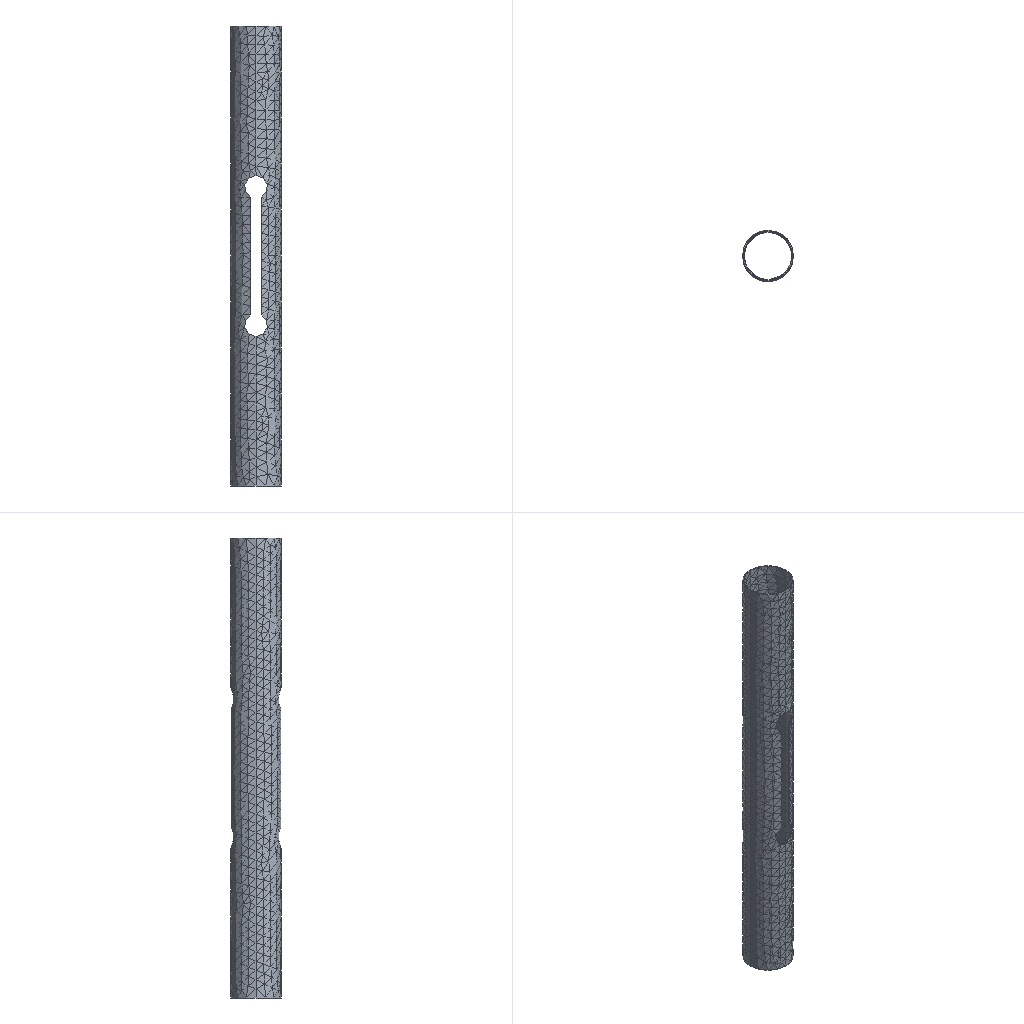Simulation study | abaqus
Set-up summary:
category,name,step,type,value,unit,region
solver,abaqus,,Abaqus/CAE 2024
units,mm-N-s-tonne (MPa),,inferred,E=210000 density=7.85e-09
analysis,Pinch_Step,,dynamic explicit,nlgeom=True; time_period=0.01
mesh,nodes,,,2587
mesh,elements,,,5865
element_type,C3D4,,,5022
element_type,R3D4,,,795
element_type,R3D3,,,48
material,Material-1,,E,210000
material,Material-1,,nu,0.3
material,Material-1,,density,7.85e-09
material,Material-1,,yield,1000
material,Material-1,,behaviors,plastic
section,Material-1,,solid section,,,Set-11
bc,BC-Deploy,Pinch_Step,fixed,"[dofs=x,y n=2]",,Set-9
bc,BC-Pinch_niehe,Pinch_Step,displacement,-60 [dofs=x],,Set-5
bc,BC-Pinch_niehe,Pinch_Step,fixed,"[dofs=rx,ry,rz,y,z n=5]",,Set-5
contact,Int-2,initial,general contact,interaction=IntProp-1; friction=0; behavior=hard
contact,Int-1,Pinch_Step,contact pair,interaction=IntProp-1; friction=0; behavior=hard,,jiaolian-waibiaomian / xinban-waibiaomian
constraint,rigid body,,,1
Abaqus input file, long lists of numbers shortened:
*Heading
** Job name: deck Model name: yuanjiaolian-Copy
** Generated by: Abaqus/CAE 2024
*Preprint, echo=NO, model=NO, history=NO, contact=NO
**
** PARTS
**
*Part, name=jiaolian11
*Node
      1, -2.39031069e-05,         -5.5,         100.
      2, -2.45171304e-05,        -5.25,         100.
** (1765 more lines like these left out)
*Element, type=C3D4
   1, 1763,  733,  592,   88
   2, 1763,   88,    6,   89
** (5020 more lines like these left out)
*Nset, nset=Set-11, generate
    1,  1767,     1
*Elset, elset=Set-11, generate
    1,  5022,     1
** Section: Section-2
*Solid Section, elset=Set-11, material=Material-1
,
*End Part
**
*Part, name=xinbang
*End Part
**
**
** ASSEMBLY
**
*Assembly, name=Assembly
**
*Instance, name=jiaolian11-1, part=jiaolian11
*End Instance
**
*Instance, name=xinbang-1, part=xinbang
          8.,          25.,          50.
          8.,          25.,          50., 8.577, 25.577, 49.423,         120.
*Node
      1,   1.961, -0.3922,          50.
      2,   1.961, -0.3922,           0.
** (817 more lines like these left out)
*Element, type=R3D4
  1,   1,   8,  41,  48
  2,   8,   9,  42,  41
** (793 more lines like these left out)
*Element, type=R3D3
257, 681, 680, 707
258, 414, 415, 382
** (46 more lines like these left out)
*Node
    820, -0.000752, 0.000577,          25.
*Nset, nset=xinbang-1-RefPt_, internal
820,
*Elset, elset=xinbang-1, generate
   1,  843,    1
*End Instance
**
*Nset, nset=Set-3, instance=jiaolian11-1
    1,    4,    9,   11,   15,   20,   23,   28,   29,   31,   33,   34,   35,   38,   56,   57
   58,   59,   60,   61,   62,   63,   64,   65,   66,   67,   68,   69,   70,  107,  108,  109
** (27 more lines like these left out)
*Elset, elset=Set-3, instance=jiaolian11-1
 2622, 2627, 2634, 2638, 2639, 2644, 2645, 2647, 2652, 2657, 2660, 2662, 2668, 2669, 2673, 2675
 2678, 2680, 2687, 2688, 2692, 2693, 2698, 2699, 2701, 2704, 2706, 2709, 2714, 2716, 2718, 2719
** (48 more lines like these left out)
*Nset, nset=Set-5, instance=xinbang-1
 820,
*Nset, nset=Set-9, instance=jiaolian11-1
   1,   2,  11,  12,  13,  14,  19,  20,  21,  22,  23,  24,  33,  34,  39,  40
 137, 138, 139, 189, 190, 191, 228, 229, 230, 231, 232, 233, 234, 235, 236, 286
** (2 more lines like these left out)
*Elset, elset=Set-9, instance=jiaolian11-1
   24,  172,  438,  439,  751,  838,  854,  856, 1019, 1180, 1185, 1195, 1199, 1204, 1207, 1211
 1213, 1386, 1388, 1395, 1802, 1855, 1876, 2048, 2076, 2077, 2080, 2089, 2091, 2094, 2100, 2102
** (4 more lines like these left out)
*Nset, nset=m_Set-6, instance=xinbang-1
 820,
*Nset, nset=_PickedSet31, internal, instance=xinbang-1
 820,
*Elset, elset=_jiaolian-waibiaomian_S2, internal, instance=jiaolian11-1
 2657, 2692, 2699, 2709, 2716, 2744, 2748, 2780, 2909, 2924, 2937, 2946, 2951, 2964, 2983, 3002
 3018, 3055, 3093, 3094, 3127, 3134, 3140, 3147, 3155, 3167, 3182, 3283, 3301, 3327, 3328, 3340
** (4 more lines like these left out)
*Elset, elset=_jiaolian-waibiaomian_S3, internal, instance=jiaolian11-1
 2622, 2644, 2647, 2652, 2662, 2668, 2673, 2675, 2678, 2687, 2688, 2701, 2704, 2706, 2718, 2719
 2721, 2722, 2754, 2756, 2757, 2758, 2767, 2768, 2771, 2773, 2774, 2779, 2782, 2788, 2795, 2806
** (27 more lines like these left out)
*Elset, elset=_jiaolian-waibiaomian_S4, internal, instance=jiaolian11-1
 2660, 2669, 2698, 2714, 2734, 2735, 2829, 2850, 2857, 2864, 2871, 2874, 2894, 2899, 2900, 2973
 3014, 3027, 3029, 3042, 3060, 3085, 3094, 3112, 3114, 3121, 3124, 3156, 3183, 3202, 3253, 3298
** (7 more lines like these left out)
*Elset, elset=_jiaolian-waibiaomian_S1, internal, instance=jiaolian11-1
 2627, 2634, 2638, 2639, 2645, 2680, 2693, 2736, 2775, 2799, 2805, 2815, 2817, 2831, 2885, 2972
 2994, 3061, 3070, 3082, 3090, 3096, 3238, 3275, 3279, 3320, 3376, 3391, 3393, 3398, 3464, 3505
** (5 more lines like these left out)
*Surface, type=ELEMENT, name=jiaolian-waibiaomian
_jiaolian-waibiaomian_S2, S2
_jiaolian-waibiaomian_S3, S3
_jiaolian-waibiaomian_S4, S4
_jiaolian-waibiaomian_S1, S1
*Elset, elset=_m_Surf-1_SPOS, internal, instance=xinbang-1, generate
 257,  808,    1
*Surface, type=ELEMENT, name=m_Surf-1
_m_Surf-1_SPOS, SPOS
*Elset, elset=_s_Surf-1_S2, internal, instance=jiaolian11-1
 2657, 2692, 2699, 2709, 2716, 2744, 2748, 2780, 2909, 2924, 2937, 2946, 2951, 2964, 2983, 3002
 3018, 3055, 3093, 3094, 3127, 3134, 3140, 3147, 3155, 3167, 3182, 3283, 3301, 3327, 3328, 3340
** (4 more lines like these left out)
*Elset, elset=_s_Surf-1_S3, internal, instance=jiaolian11-1
 2622, 2644, 2647, 2652, 2662, 2668, 2673, 2675, 2678, 2687, 2688, 2701, 2704, 2706, 2718, 2719
 2721, 2722, 2754, 2756, 2757, 2758, 2767, 2768, 2771, 2773, 2774, 2779, 2782, 2788, 2795, 2806
** (27 more lines like these left out)
*Elset, elset=_s_Surf-1_S4, internal, instance=jiaolian11-1
 2660, 2669, 2698, 2714, 2734, 2735, 2829, 2850, 2857, 2864, 2871, 2874, 2894, 2899, 2900, 2973
 3014, 3027, 3029, 3042, 3060, 3085, 3094, 3112, 3114, 3121, 3124, 3156, 3183, 3202, 3253, 3298
** (7 more lines like these left out)
*Elset, elset=_s_Surf-1_S1, internal, instance=jiaolian11-1
 2627, 2634, 2638, 2639, 2645, 2680, 2693, 2736, 2775, 2799, 2805, 2815, 2817, 2831, 2885, 2972
 2994, 3061, 3070, 3082, 3090, 3096, 3238, 3275, 3279, 3320, 3376, 3391, 3393, 3398, 3464, 3505
** (5 more lines like these left out)
*Surface, type=ELEMENT, name=s_Surf-1
_s_Surf-1_S2, S2
_s_Surf-1_S3, S3
_s_Surf-1_S4, S4
_s_Surf-1_S1, S1
*Elset, elset=_s_Surf-3_S2, internal, instance=jiaolian11-1
 2657, 2692, 2699, 2709, 2716, 2744, 2748, 2780, 2909, 2924, 2937, 2946, 2951, 2964, 2983, 3002
 3018, 3055, 3093, 3094, 3127, 3134, 3140, 3147, 3155, 3167, 3182, 3283, 3301, 3327, 3328, 3340
** (4 more lines like these left out)
*Elset, elset=_s_Surf-3_S3, internal, instance=jiaolian11-1
 2622, 2644, 2647, 2652, 2662, 2668, 2673, 2675, 2678, 2687, 2688, 2701, 2704, 2706, 2718, 2719
 2721, 2722, 2754, 2756, 2757, 2758, 2767, 2768, 2771, 2773, 2774, 2779, 2782, 2788, 2795, 2806
** (27 more lines like these left out)
*Elset, elset=_s_Surf-3_S4, internal, instance=jiaolian11-1
 2660, 2669, 2698, 2714, 2734, 2735, 2829, 2850, 2857, 2864, 2871, 2874, 2894, 2899, 2900, 2973
 3014, 3027, 3029, 3042, 3060, 3085, 3094, 3112, 3114, 3121, 3124, 3156, 3183, 3202, 3253, 3298
** (7 more lines like these left out)
*Elset, elset=_s_Surf-3_S1, internal, instance=jiaolian11-1
 2627, 2634, 2638, 2639, 2645, 2680, 2693, 2736, 2775, 2799, 2805, 2815, 2817, 2831, 2885, 2972
 2994, 3061, 3070, 3082, 3090, 3096, 3238, 3275, 3279, 3320, 3376, 3391, 3393, 3398, 3464, 3505
** (5 more lines like these left out)
*Surface, type=ELEMENT, name=s_Surf-3
_s_Surf-3_S2, S2
_s_Surf-3_S3, S3
_s_Surf-3_S4, S4
_s_Surf-3_S1, S1
*Elset, elset=_s_Surf-6_S4, internal, instance=jiaolian11-1
   21,   25,   27,   35,   61,   70,   71,   76,   82,   88,   96,  101,  108,  118,  127,  128
  145,  151,  157,  166,  167,  171,  195,  198,  204,  207,  209,  221,  231,  241,  244,  245
** (42 more lines like these left out)
*Elset, elset=_s_Surf-6_S2, internal, instance=jiaolian11-1
    5,   18,   30,   31,   32,   33,   43,   47,   50,   53,   63,   68,   69,   78,   89,   99
  114,  122,  124,  125,  130,  135,  140,  147,  153,  156,  163,  194,  199,  210,  211,  217
** (47 more lines like these left out)
*Elset, elset=_s_Surf-6_S1, internal, instance=jiaolian11-1
   19,   29,   34,   51,   57,   65,   67,   77,   79,   94,  103,  107,  111,  117,  129,  137
  139,  143,  150,  155,  158,  160,  161,  162,  168,  172,  177,  184,  189,  196,  200,  208
** (41 more lines like these left out)
*Elset, elset=_s_Surf-6_S3, internal, instance=jiaolian11-1
   13,   16,   23,   24,   36,   37,   39,   44,   45,   52,   56,   58,   66,   72,   73,   81
   98,  102,  104,  105,  106,  109,  110,  112,  116,  119,  131,  132,  138,  142,  148,  149
** (75 more lines like these left out)
*Surface, type=ELEMENT, name=s_Surf-6
_s_Surf-6_S4, S4
_s_Surf-6_S2, S2
_s_Surf-6_S1, S1
_s_Surf-6_S3, S3
*Elset, elset=_xinban-waibiaomian_SPOS, internal, instance=xinbang-1, generate
 257,  808,    1
*Surface, type=ELEMENT, name=xinban-waibiaomian
_xinban-waibiaomian_SPOS, SPOS
*Rigid Body, ref node=xinbang-1.xinbang-1-RefPt_, elset=xinbang-1.xinbang-1
*End Assembly
*Amplitude, name=Amp-1
             0.,              0.,            0.01,              1.
**
** MATERIALS
**
*Material, name=Material-1
*Density
 7.85e-09,
*Elastic
210000., 0.3
*Plastic
1000.,0.
**
** INTERACTION PROPERTIES
**
*Surface Interaction, name=IntProp-1
*Friction
0.,
*Surface Behavior, pressure-overclosure=HARD
**
** INTERACTIONS
**
** Interaction: Int-2
*Contact, op=NEW
*Contact Inclusions, ALL EXTERIOR
*Contact Property Assignment
 ,  , IntProp-1
** ----------------------------------------------------------------
**
** STEP: Pinch_Step
**
*Step, name=Pinch_Step, nlgeom=YES
*Dynamic, Explicit
, 0.01
*Bulk Viscosity
0.06, 1.2
** Mass Scaling: Semi-Automatic
**               Whole Model
*Fixed Mass Scaling, factor=10000.
**
** BOUNDARY CONDITIONS
**
** Name: BC-Deploy Type: Displacement/Rotation
*Boundary
Set-9, 1, 1
Set-9, 2, 2
** Name: BC-Pinch_niehe Type: Displacement/Rotation
*Boundary, amplitude=Amp-1
Set-5, 1, 1, -60.
Set-5, 2, 2
Set-5, 3, 3
Set-5, 4, 4
Set-5, 5, 5
Set-5, 6, 6
**
** INTERACTIONS
**
** Interaction: Int-1
*Contact Pair, interaction=IntProp-1, mechanical constraint=KINEMATIC, cpset=Int-1
jiaolian-waibiaomian, xinban-waibiaomian
**
** OUTPUT REQUESTS
**
*Restart, write, number interval=1, time marks=NO
**
** FIELD OUTPUT: F-Output-1
**
*Output, field, variable=PRESELECT
**
** HISTORY OUTPUT: H-Output-1
**
*Output, history, variable=PRESELECT, frequency=1
*End Step
Results summary:
result,odb.job_status,,,JOB_STATUS_COMPLETED_SUCCESSFULLY,"consistent, unstated (Abaqus has no unit system)"
result,steps[0].procedure,Pinch_Step,,"*DYNAMIC, EXPLICIT","consistent, unstated (Abaqus has no unit system)"
result,steps[0].time_period,Pinch_Step,,0.01,"consistent, unstated (Abaqus has no unit system)"
result,steps[0].n_frames,Pinch_Step,,21,"consistent, unstated (Abaqus has no unit system)"
result,steps[0].last_frame.id,Pinch_Step,,8378,"consistent, unstated (Abaqus has no unit system)"
result,steps[0].last_frame.value,Pinch_Step,,0.01,"consistent, unstated (Abaqus has no unit system)"
result,steps[0].last_frame.description,Pinch_Step,,Increment      8378: Step Time =   1.0000E-02,"consistent, unstated (Abaqus has no unit system)"
result,steps[0].completed,Pinch_Step,,True,"consistent, unstated (Abaqus has no unit system)"
result,steps[0].max_U_magnitude,Pinch_Step,,60.379,"consistent, unstated (Abaqus has no unit system)"
result,steps[0].max_S_mises,Pinch_Step,,1000.01,"consistent, unstated (Abaqus has no unit system)"
result,steps[0].RF_sum[1],Pinch_Step,,-9322.55,"consistent, unstated (Abaqus has no unit system)"
result,steps[0].RF_sum[2],Pinch_Step,,250.907,"consistent, unstated (Abaqus has no unit system)"
result,steps[0].RF_sum[3],Pinch_Step,,-2036.43,"consistent, unstated (Abaqus has no unit system)"
result,steps[0].diagnostic.n_increments,Pinch_Step,,21,"consistent, unstated (Abaqus has no unit system)"